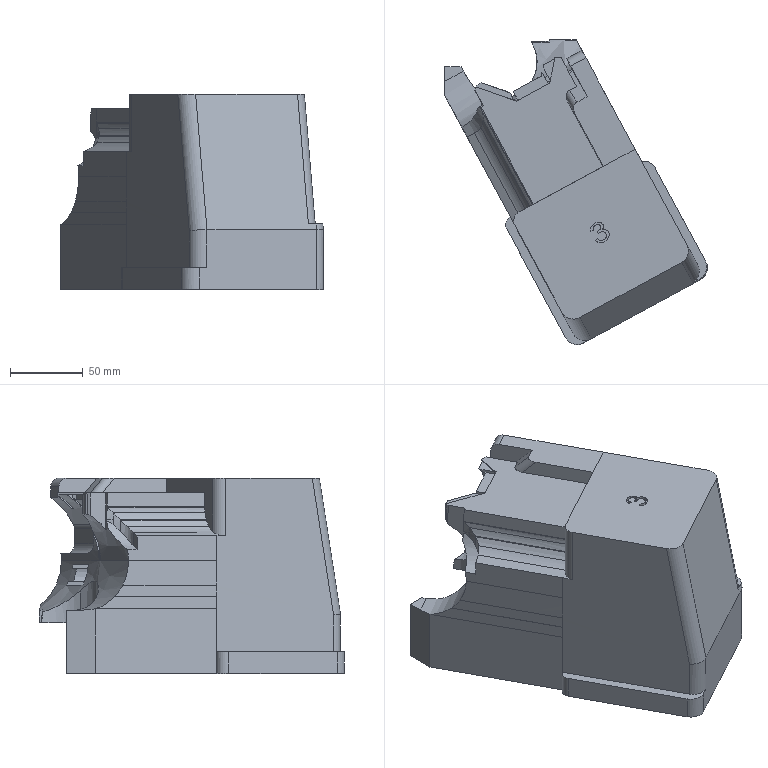Part | Creo | 1 solid | 166 faces | box 180.536 x 209.471 x 134.083 mm | volume 1992064 mm3 | plane 90 | cylinder 43 | other 18 | cone 9 | spline 6 | commonest cylinder face diameters 18 x8 13.054 x3 8.042 x2 32.163 x2 49.623 x2 58.774 x2